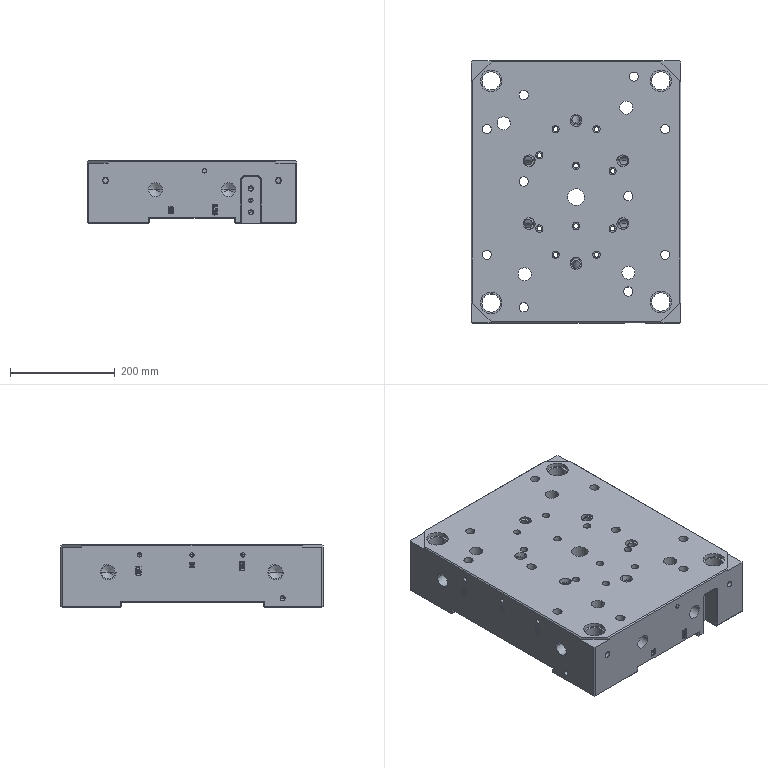Part | Creo | 1 solid | 1958 faces | box 400 x 500 x 120 mm | volume 15409066 mm3 | plane 761 | cylinder 502 | other 365 | cone 306 | spline 20 | torus 4 | commonest cylinder face diameters 6 x88 4.97 x60 8 x60 5 x32 14 x28 6.71 x20